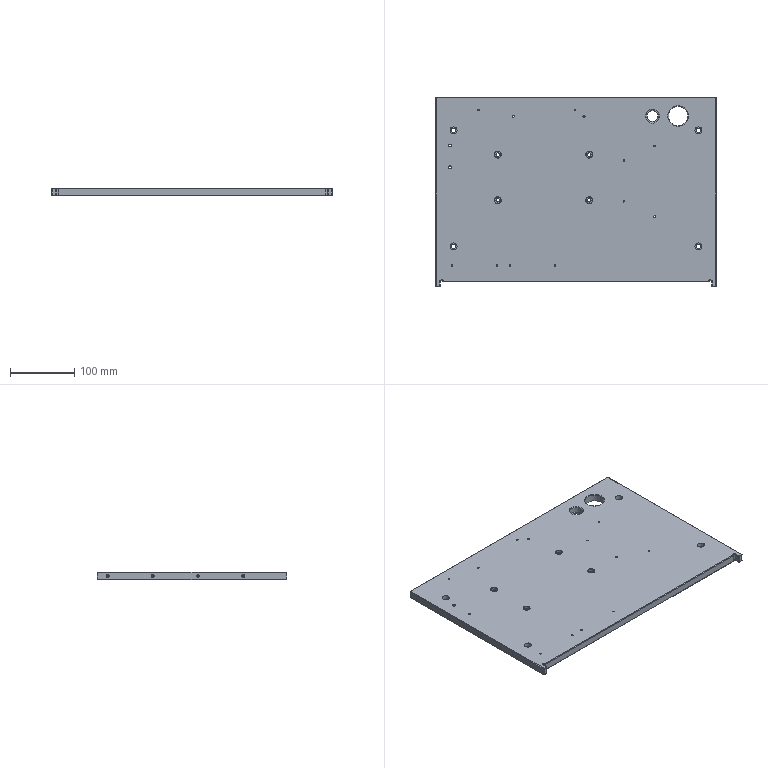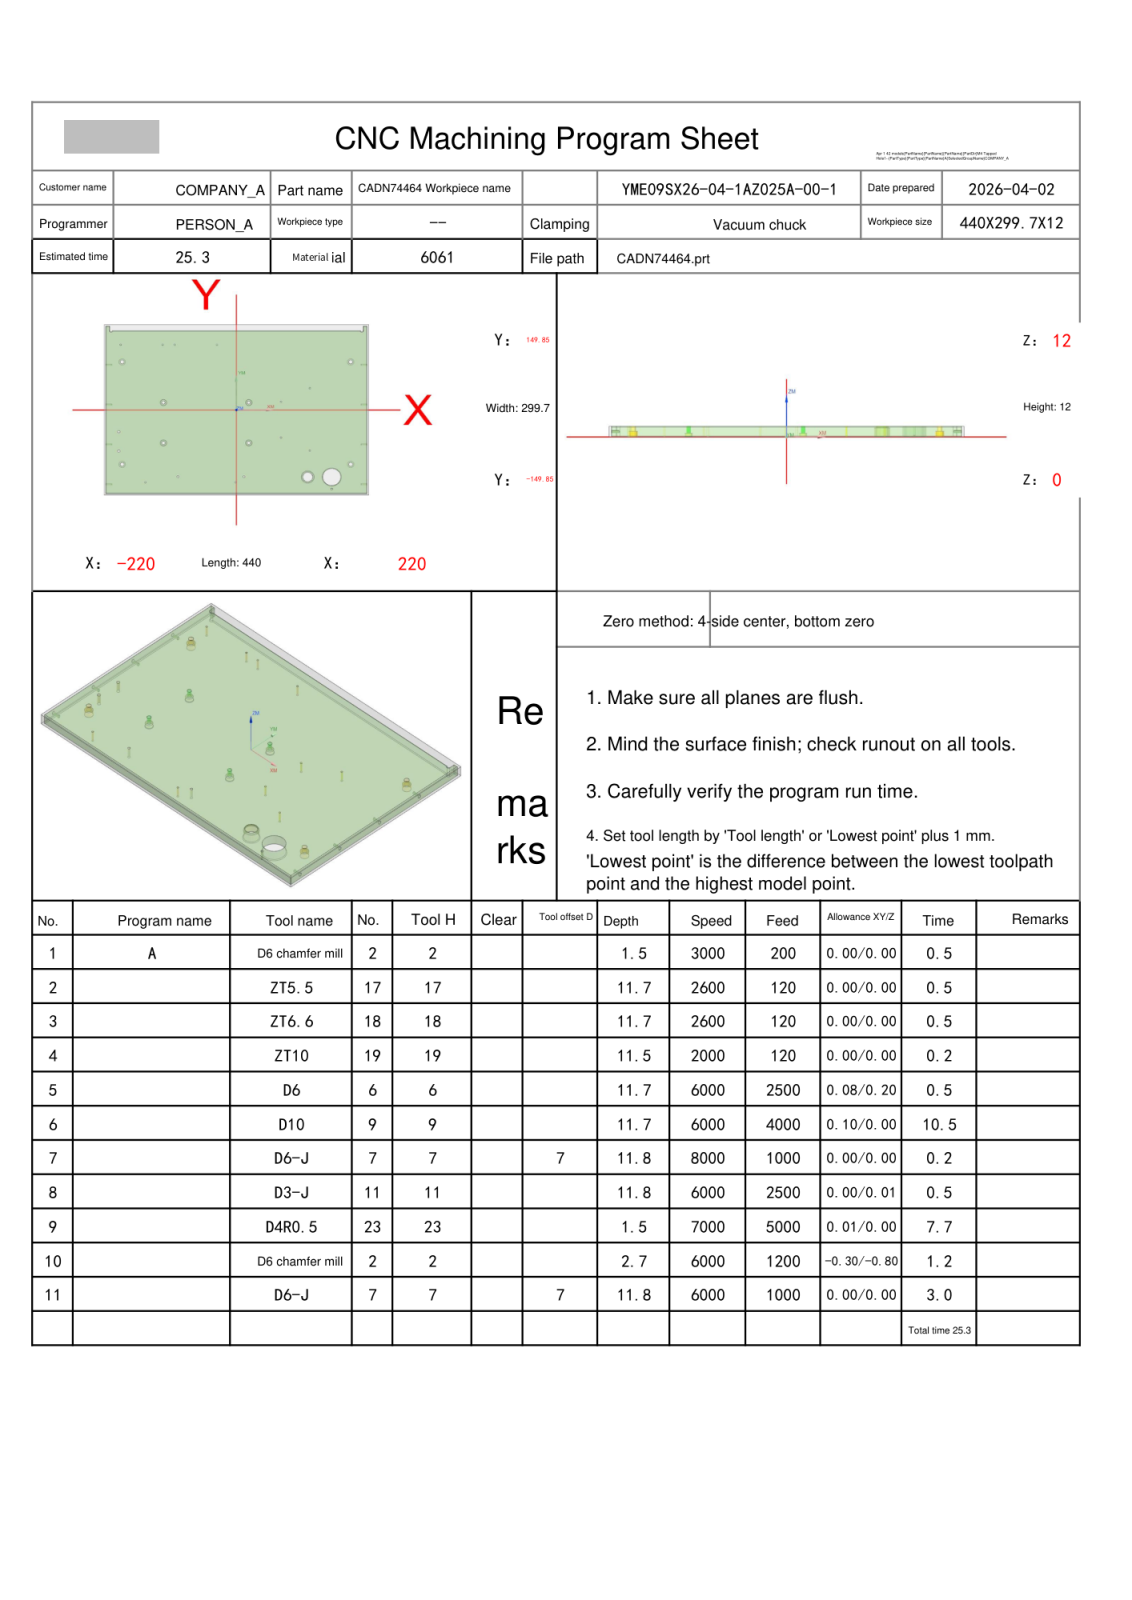NC program | NX | posted by the shop | part box 435 x 294.7 x 12 mm
Lines 23830 to 24066 of 24066:
N10 T02 M06
(D6 chamfer mill  D=6. R=0. H=02 ce=0.00 di=0.00)
G00 G90 G54 X112.363 Y-117.557 M03 S6000
G43 H02 Z32.
M08
Z14.131
G01 Z10.501 F1200.
G03 X112.091 Y-117.492 I-.272 J-.535
X111.556 Y-117.82 I0.0 J-.6
G01 X111.55 Y-117.85
G03 X118.5 Y-124.8 I6.95 J0.0
X125.45 Y-117.85 I0.0 J6.95
X118.5 Y-110.9 I-6.95 J0.0
X111.55 Y-117.85 I0.0 J-6.95
G01 X111.556 Y-117.88
G03 X112.091 Y-118.208 I.535 J.272
X112.363 Y-118.143 I0.0 J.6
G01 Z14.131
G00 Z32.
X145.618 Y-117.57
Z14.119
G01 Z10.501
G03 X145.337 Y-117.5 I-.28 J-.53
X144.807 Y-117.82 I0.0 J-.6
G01 X144.8 Y-117.85
G03 X158.5 Y-131.55 I13.7 J0.0
X172.2 Y-117.85 I0.0 J13.7
X158.5 Y-104.15 I-13.7 J0.0
X144.8 Y-117.85 I0.0 J-13.7
G01 X144.807 Y-117.88
G03 X145.337 Y-118.2 I.53 J.28
X145.618 Y-118.13 I0.0 J.6
G01 Z14.119
G00 Z32.
G00 G90 X-151.5 Y-127.35 M03 S5000
Z32.
G98 G81 X-151.5 Y-127.35 Z10.25 R15. F150.
X-1.5
X74.218 Y-48.701
X121.901 Y-71.329
Y38.171
X74.218 Y14.299
X-32.5 Y114.35
X-102.5
X-122.5
X-192.5
G80
G00 Z32.
G00 G90 X158.5 Y-138.85 M03 S5000
Z32.
G98 G81 X158.5 Y-138.85 Z9.8 R15. F150.
X12.5 Y-117.35
X-97.5
G80
G00 Z32.
G00 G90 X-195.5 Y-72.35 M03 S5000
Z32.
G98 G81 X-195.5 Y-72.35 Z9.3 R15. F150.
Y-38.35
G80
G00 Z32.
G00 G90 X20.51 Y-57.462 M03 S6000
Z32.
Z11.1
G01 Z10.6 F600.
X20.425 Y-56.609
G03 X18.925 Y-58.109 I0.0 J-1.5
X20.575 Y-59.759 I1.65 J0.0
X22.225 Y-58.109 I0.0 J1.65
X20.575 Y-56.459 I-1.65 J0.0
X18.925 Y-58.109 I0.0 J-1.65
X20.425 Y-59.609 I1.5 J0.0
G01 X20.51 Y-58.756
Z11.1
G00 Z32.
Y13.538
Z11.1
G01 Z10.6
X20.425 Y14.391
G03 X18.925 Y12.891 I0.0 J-1.5
X20.575 Y11.241 I1.65 J0.0
X22.225 Y12.891 I0.0 J1.65
X20.575 Y14.541 I-1.65 J0.0
X18.925 Y12.891 I0.0 J-1.65
X20.425 Y11.391 I1.5 J0.0
G01 X20.51 Y12.244
Z11.1
G00 Z32.
X-121.49 Y13.538
Z11.1
G01 Z10.6
X-121.575 Y14.391
G03 X-123.075 Y12.891 I0.0 J-1.5
X-121.425 Y11.241 I1.65 J0.0
X-119.775 Y12.891 I0.0 J1.65
X-121.425 Y14.541 I-1.65 J0.0
X-123.075 Y12.891 I0.0 J-1.65
X-121.575 Y11.391 I1.5 J0.0
G01 X-121.49 Y12.244
Z11.1
G00 Z32.
Y-57.462
Z11.1
G01 Z10.6
X-121.575 Y-56.609
G03 X-123.075 Y-58.109 I0.0 J-1.5
X-121.425 Y-59.759 I1.65 J0.0
X-119.775 Y-58.109 I0.0 J1.65
X-121.425 Y-56.459 I-1.65 J0.0
X-123.075 Y-58.109 I0.0 J-1.65
X-121.575 Y-59.609 I1.5 J0.0
G01 X-121.49 Y-58.756
Z11.1
G00 Z32.
G00 G90 X189.493 Y85.434 M03 S6000
Z32.
Z11.1
G01 Z10.6 F600.
X189.3 Y85.846
G03 X187.8 Y84.346 I0.0 J-1.5
X190. Y82.146 I2.2 J0.0
X192.2 Y84.346 I0.0 J2.2
X190. Y86.546 I-2.2 J0.0
X187.8 Y84.346 I0.0 J-2.2
X189.3 Y82.846 I1.5 J0.0
G01 X189.493 Y83.259
Z11.1
G00 Z32.
Y-94.566
Z11.1
G01 Z10.6
X189.3 Y-94.154
G03 X187.8 Y-95.654 I0.0 J-1.5
X190. Y-97.854 I2.2 J0.0
X192.2 Y-95.654 I0.0 J2.2
X190. Y-93.454 I-2.2 J0.0
X187.8 Y-95.654 I0.0 J-2.2
X189.3 Y-97.154 I1.5 J0.0
G01 X189.493 Y-96.741
Z11.1
G00 Z32.
X-190.507 Y-94.566
Z11.1
G01 Z10.6
X-190.7 Y-94.154
G03 X-192.2 Y-95.654 I0.0 J-1.5
X-190. Y-97.854 I2.2 J0.0
X-187.8 Y-95.654 I0.0 J2.2
X-190. Y-93.454 I-2.2 J0.0
X-192.2 Y-95.654 I0.0 J-2.2
X-190.7 Y-97.154 I1.5 J0.0
G01 X-190.507 Y-96.741
Z11.1
G00 Z32.
Y85.434
Z11.1
G01 Z10.6
X-190.7 Y85.846
G03 X-192.2 Y84.346 I0.0 J-1.5
X-190. Y82.146 I2.2 J0.0
X-187.8 Y84.346 I0.0 J2.2
X-190. Y86.546 I-2.2 J0.0
X-192.2 Y84.346 I0.0 J-2.2
X-190.7 Y82.846 I1.5 J0.0
G01 X-190.507 Y83.259
Z11.1
G00 Z32.
G91 G28 Z0.0
M05
M09
G91 G28 Z0.0
M01
N11 T07 M06
(D6-J  D=6. R=0. H=07 ce=0.00 di=0.00)
G00 G90 G54 X217.515 Y-151.449 M03 S6000
G43 H07 Z32.
M08
Z1.
G01 Z.5 F1000.
G41 D07
X217.495 Y-151.25
G03 X216.5 Y-150.35 I-.995 J-.1
G01 X-216.5
G02 X-220.5 Y-146.35 I0.0 J4.
G01 Y146.35
G02 X-216.5 Y150.35 I4. J0.0
G01 X-211.5
G02 X-207.5 Y146.35 I0.0 J-4.
G01 Y142.178
G02 X-206.5 Y142.35 I1. J-2.828
G01 X206.5
G02 X207.5 Y142.178 I0.0 J-3.
G01 Y146.35
G02 X211.5 Y150.35 I4. J0.0
G01 X216.5
G02 X220.5 Y146.35 I0.0 J-4.
G01 Y-146.35
G02 X216.5 Y-150.35 I-4. J0.0
G01 X216.
G03 X215. Y-151.35 I0.0 J-1.
G01 G40 Y-151.55
Z1.
G00 Z32.
G00 G90 X217.505 Y-151.349 M03 S6000
Z32.
Z.7
G01 Z.2 F1000.
G41 D07
X217.495 Y-151.25
G03 X216.5 Y-150.35 I-.995 J-.1
G01 X-216.5
G02 X-220.5 Y-146.35 I0.0 J4.
G01 Y146.35
G02 X-216.5 Y150.35 I4. J0.0
G01 X-211.5
G02 X-207.5 Y146.35 I0.0 J-4.
G01 Y142.178
G02 X-206.5 Y142.35 I1. J-2.828
G01 X206.5
G02 X207.5 Y142.178 I0.0 J-3.
G01 Y146.35
G02 X211.5 Y150.35 I4. J0.0
G01 X216.5
G02 X220.5 Y146.35 I0.0 J-4.
G01 Y-146.35
G02 X216.5 Y-150.35 I-4. J0.0
G01 X216.
G03 X215. Y-151.35 I0.0 J-1.
G01 G40 Y-151.45
Z.7
G00 Z32.
M05
M09
G91 G28 Z0.0
G91 G28 Y0.0
M30
%